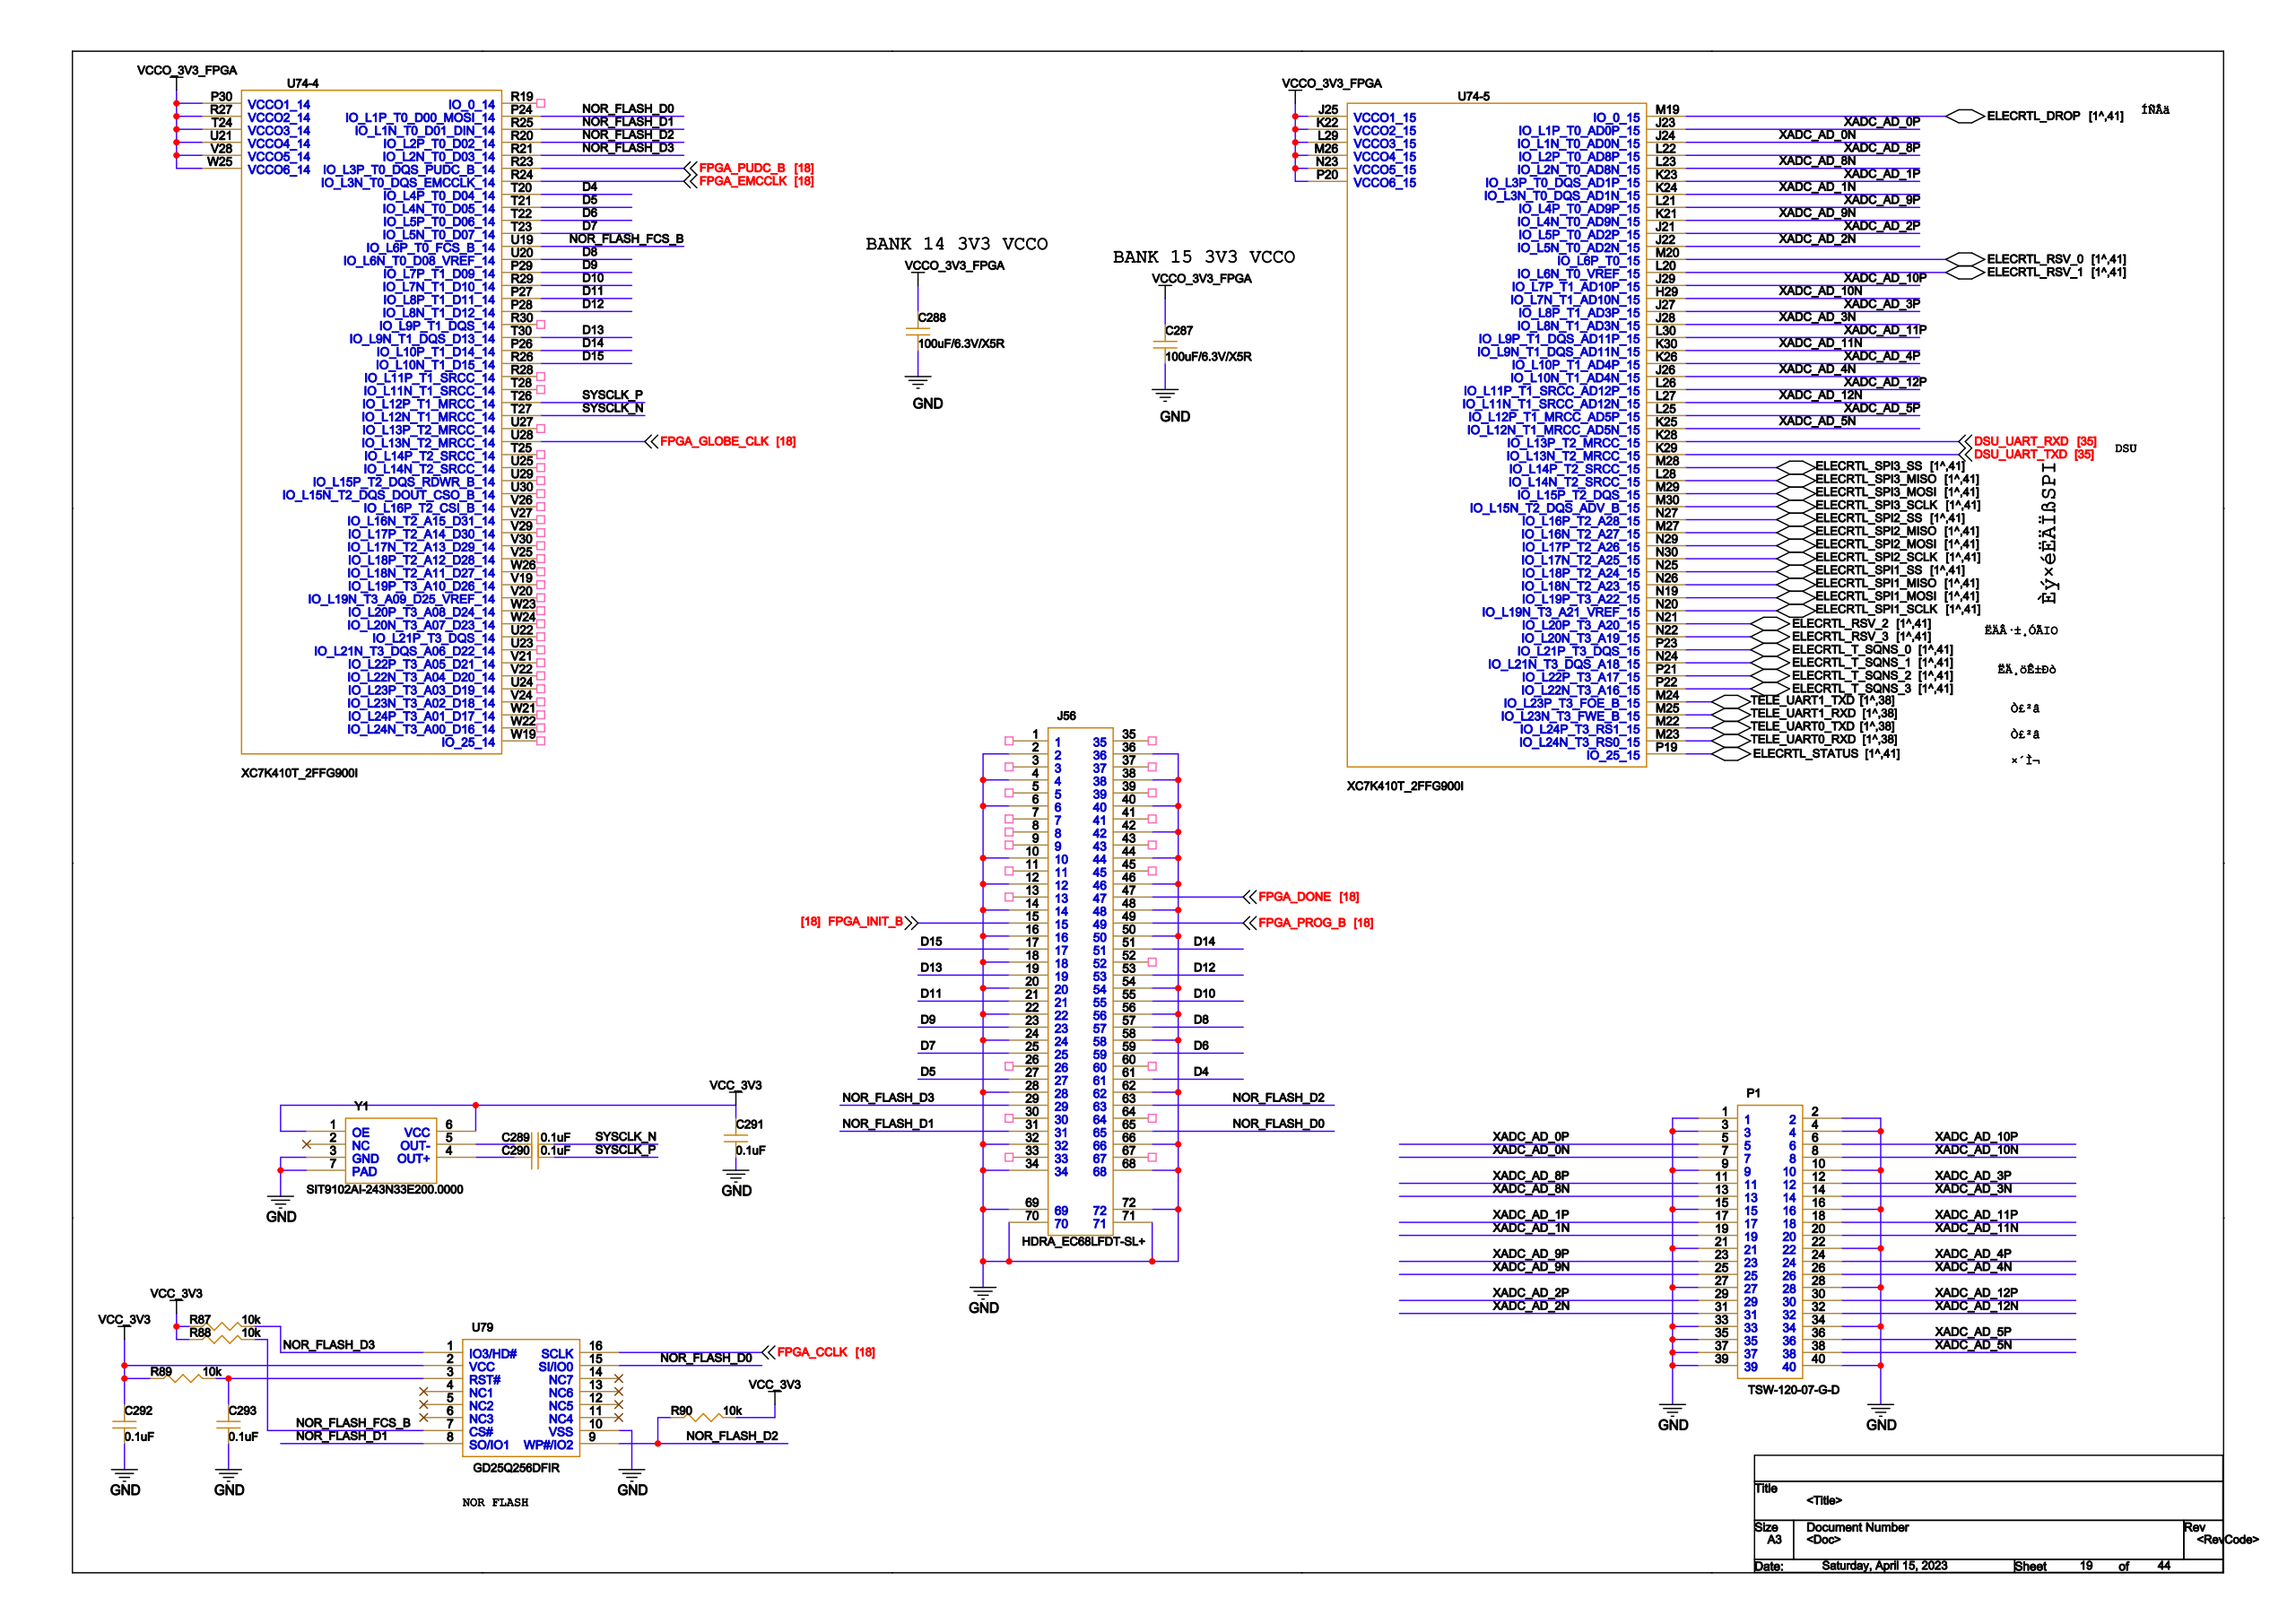Circuit board | Cadence Allegro | 1034 parts | 912 nets | one sheet of the schematic
Parts on this sheet (reference | value | footprint):
C287 | 100uF/6.3V/X5R | C0402_BGA
C288 | 100uF/6.3V/X5R | C0402_BGA
C289 | 0.1uF | C0402
C290 | 0.1uF | C0402
C291 | 0.1uF | C0402
C292 | 0.1uF | C0402
C293 | 0.1uF | C0402
J56 | HDRA_EC68LFDT-SL+ | HDRA_EC68LFDT-SL
P1 | TSW-120-07-G-D | TSW_2MM54_DR
R87 | 10k | R0402
R88 | 10k | R0402
R89 | 10k | R0402
R90 | 10k | R0402
U79 | GD25Q256DFIR | SOP16-1_27-10_3X10_3
Y1 | SIT9102AI-243N33E200 | SIT_7MM0X5MM0
Nets of these parts (net: part-pin ...):
GND: C287-1 C288-1 C291-1 C292-1 C293-1 U79-10 Y1-3 Y1-7 J56-2 J56-4 J56-6 J56-10 J56-12 J56-14 J56-16 J56-18 J56-20 J56-22 J56-24 J56-28 J56-32 J56-34 J56-36 J56-38 J56-40 J56-42 J56-44 J56-46 J56-48 J56-50 J56-54 J56-56 J56-58 J56-62 J56-66 J56-68 J56-69 J56-70 J56-71 J56-72 P1-1 P1-2 P1-3 P1-4 P1-9 P1-10 P1-15 P1-16 P1-21 P1-22 P1-27 P1-28 P1-33 P1-34 P1-35 P1-37 P1-39 P1-40
VCC_3V3: C291-2 C292-2 R87-1 R88-1 R89-1 R90-2 U79-2 Y1-1 Y1-6
VCCO_3V3_FPGA: C287-2 C288-2
N13933384: C293-2 R89-2 U79-3
SYSCLK_N: C289-1
N14074961: C289-2 Y1-5
SYSCLK_P: C290-1
N14074959: C290-2 Y1-4
FPGA_PROG_B: J56-49
FPGA_CCLK: U79-16
FPGA_INIT_B: J56-15
D15: J56-17
D13: J56-19
D11: J56-21
D9: J56-23
D7: J56-25
D5: J56-27
NOR_FLASH_D3: R87-2 U79-1 J56-29
NOR_FLASH_D1: U79-8 J56-31
FPGA_DONE: J56-47
D14: J56-51
D12: J56-53
D10: J56-55
D8: J56-57
D6: J56-59
D4: J56-61
NOR_FLASH_D2: R90-1 U79-9 J56-63
NOR_FLASH_D0: U79-15 J56-65
XADC_AD_8P: P1-11
XADC_AD_3P: P1-12
XADC_AD_8N: P1-13
XADC_AD_3N: P1-14
XADC_AD_1P: P1-17
XADC_AD_11P: P1-18
XADC_AD_1N: P1-19
XADC_AD_11N: P1-20
XADC_AD_9P: P1-23
XADC_AD_4P: P1-24
XADC_AD_9N: P1-25
XADC_AD_4N: P1-26
XADC_AD_2P: P1-29
XADC_AD_12P: P1-30
XADC_AD_2N: P1-31
XADC_AD_12N: P1-32
XADC_AD_5P: P1-36
XADC_AD_5N: P1-38
XADC_AD_0P: P1-5
XADC_AD_10P: P1-6
XADC_AD_0N: P1-7
XADC_AD_10N: P1-8
NOR_FLASH_FCS_B: R88-2 U79-7